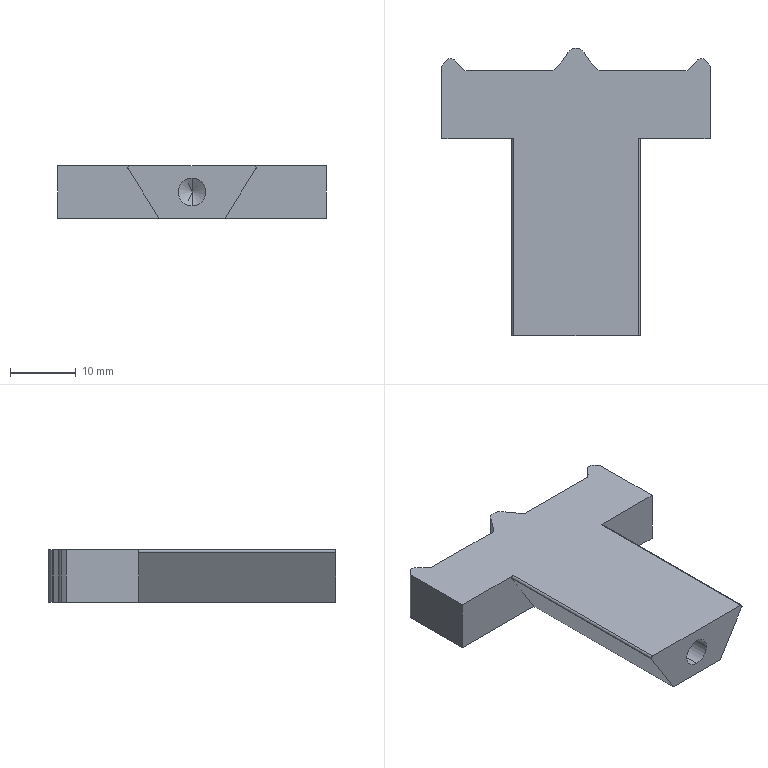Part | STEP file | positioning fork | 1 solid | 28 faces | box 40.8 x 43.762 x 8 mm | volume 6960 mm3 | plane 15 | cylinder 11 | cone 2 | commonest cylinder face diameters 20.4 x4 0.6 x2 2 x2 4.2 x2 3 x1